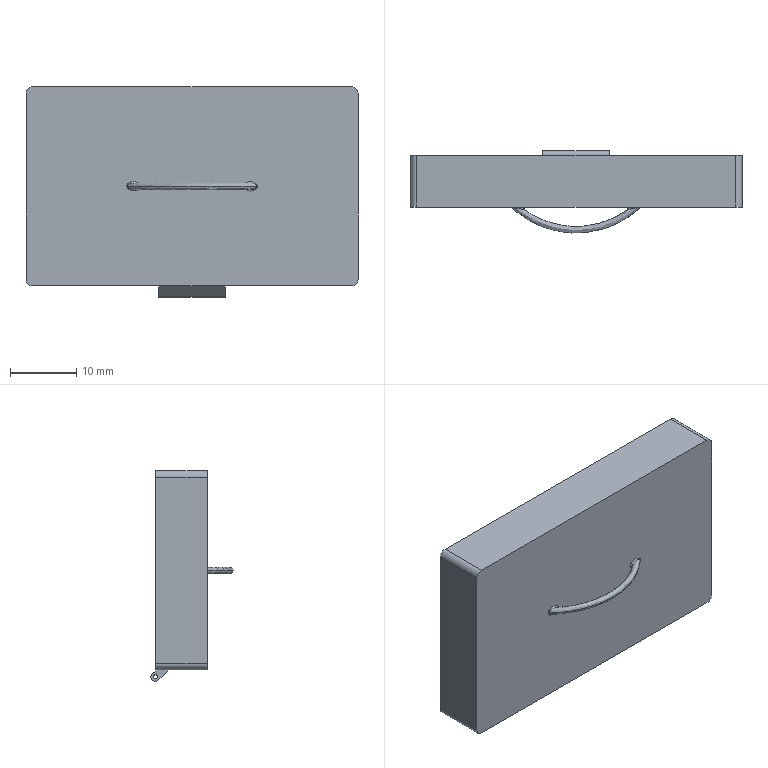Part | SolidWorks | features Fillet 2, ICE 2, BossThin 1, Extrusion 1, Shell 1, Sweep 1 | 1 solid | 32 faces | box 50 x 12.396 x 31.7 mm | volume 2667 mm3 | plane 19 | cylinder 7 | spline 6 | commonest cylinder face diameters 2 x4 0.6 x2 1.4 x1